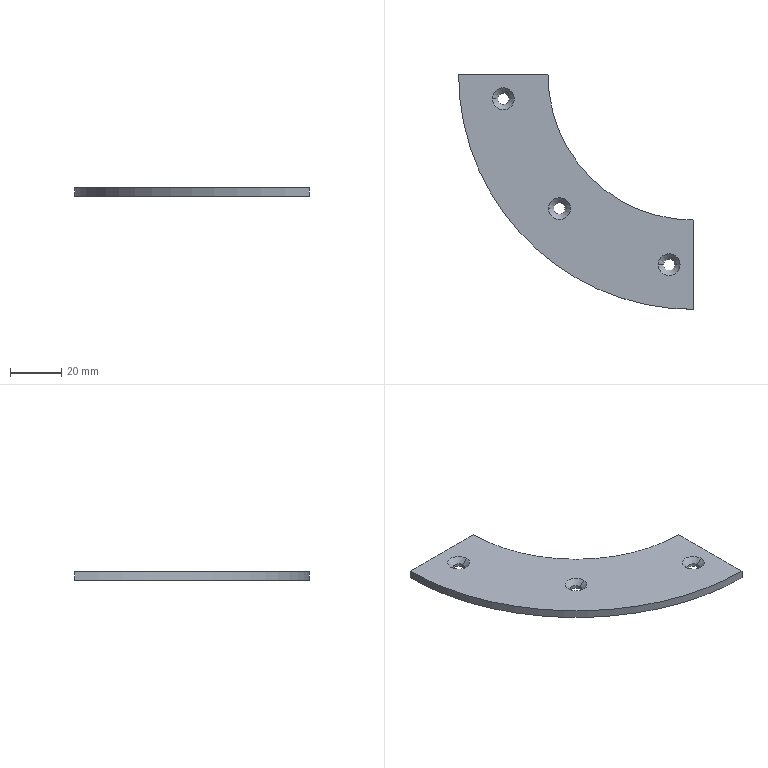Part | SolidWorks | features BaseBody 1 | 1 solid | 18 faces | box 92 x 92 x 3.2 mm | volume 12838 mm3 | cylinder 8 | cone 6 | plane 4 | commonest cylinder face diameters 4.5 x6 114 x1 184 x1
STEP:
#1=CARTESIAN_POINT('',(-50.25,-52.5,-3.2));
#2=VERTEX_POINT('',#1);
#3=CARTESIAN_POINT('',(-54.75,-52.5,-3.2));
#4=VERTEX_POINT('',#3);
#5=CARTESIAN_POINT('',(-52.5,-52.5,-3.2));
#6=DIRECTION('',(0.,0.,-1.));
#7=DIRECTION('',(1.,0.,0.));
#8=AXIS2_PLACEMENT_3D('',#5,#6,#7);
#9=CIRCLE('',#8,2.25);
#10=EDGE_CURVE('',#2,#4,#9,.T.);
#11=ORIENTED_EDGE('',*,*,#10,.T.);
#12=CARTESIAN_POINT('',(-54.75,-52.5,-2.05));
#13=VERTEX_POINT('',#12);
#14=CARTESIAN_POINT('',(-54.75,-52.5,0.));
#15=DIRECTION('',(0.,0.,1.));
#16=VECTOR('',#15,1000.);
#17=LINE('',#14,#16);
#18=EDGE_CURVE('',#4,#13,#17,.T.);
#19=ORIENTED_EDGE('',*,*,#18,.T.);
#20=CARTESIAN_POINT('',(-50.25,-52.5,-2.05));
#21=VERTEX_POINT('',#20);
#22=CARTESIAN_POINT('',(-52.5,-52.5,-2.05));
#23=DIRECTION('',(0.,0.,-1.));
#24=DIRECTION('',(1.,0.,0.));
#25=AXIS2_PLACEMENT_3D('',#22,#23,#24);
#26=CIRCLE('',#25,2.25);
#27=EDGE_CURVE('',#21,#13,#26,.T.);
#28=ORIENTED_EDGE('',*,*,#27,.F.);
#29=CARTESIAN_POINT('',(-50.25,-52.5,0.));
#30=DIRECTION('',(0.,0.,1.));
#31=VECTOR('',#30,1000.);
#32=LINE('',#29,#31);
#33=EDGE_CURVE('',#2,#21,#32,.T.);
#34=ORIENTED_EDGE('',*,*,#33,.F.);
#35=EDGE_LOOP('',(#11,#19,#28,#34));
#36=FACE_OUTER_BOUND('',#35,.T.);
#37=CARTESIAN_POINT('',(-52.5,-52.5,0.));
#38=DIRECTION('',(0.,0.,1.));
#39=DIRECTION('',(1.,0.,0.));
#40=AXIS2_PLACEMENT_3D('',#37,#38,#39);
#41=CYLINDRICAL_SURFACE('',#40,2.25);
#42=ADVANCED_FACE('',(#36),#41,.F.);
#43=CARTESIAN_POINT('',(-72.25,-9.5,-3.2));
#44=VERTEX_POINT('',#43);
#45=CARTESIAN_POINT('',(-76.75,-9.5,-3.2));
#46=VERTEX_POINT('',#45);
#47=CARTESIAN_POINT('',(-74.5,-9.5,-3.2));
#48=DIRECTION('',(0.,0.,-1.));
#49=DIRECTION('',(1.,0.,0.));
#50=AXIS2_PLACEMENT_3D('',#47,#48,#49);
#51=CIRCLE('',#50,2.25);
#52=EDGE_CURVE('',#44,#46,#51,.T.);
#53=ORIENTED_EDGE('',*,*,#52,.T.);
#54=CARTESIAN_POINT('',(-76.75,-9.5,-2.05));
#55=VERTEX_POINT('',#54);
#56=CARTESIAN_POINT('',(-76.75,-9.5,0.));
#57=DIRECTION('',(0.,0.,1.));
#58=VECTOR('',#57,1000.);
#59=LINE('',#56,#58);
#60=EDGE_CURVE('',#46,#55,#59,.T.);
#61=ORIENTED_EDGE('',*,*,#60,.T.);
#62=CARTESIAN_POINT('',(-72.25,-9.5,-2.05));
#63=VERTEX_POINT('',#62);
#64=CARTESIAN_POINT('',(-74.5,-9.5,-2.05));
#65=DIRECTION('',(0.,0.,-1.));
#66=DIRECTION('',(1.,0.,0.));
#67=AXIS2_PLACEMENT_3D('',#64,#65,#66);
#68=CIRCLE('',#67,2.25);
#69=EDGE_CURVE('',#63,#55,#68,.T.);
#70=ORIENTED_EDGE('',*,*,#69,.F.);
#71=CARTESIAN_POINT('',(-72.25,-9.5,0.));
#72=DIRECTION('',(0.,0.,1.));
#73=VECTOR('',#72,1000.);
#74=LINE('',#71,#73);
#75=EDGE_CURVE('',#44,#63,#74,.T.);
#76=ORIENTED_EDGE('',*,*,#75,.F.);
#77=EDGE_LOOP('',(#53,#61,#70,#76));
#78=FACE_OUTER_BOUND('',#77,.T.);
#79=CARTESIAN_POINT('',(-74.5,-9.5,0.));
#80=DIRECTION('',(0.,0.,1.));
#81=DIRECTION('',(1.,0.,0.));
#82=AXIS2_PLACEMENT_3D('',#79,#80,#81);
#83=CYLINDRICAL_SURFACE('',#82,2.25);
#84=ADVANCED_FACE('',(#78),#83,.F.);
#85=CARTESIAN_POINT('',(-7.25,-74.5,-3.2));
#86=VERTEX_POINT('',#85);
#87=CARTESIAN_POINT('',(-11.75,-74.5,-3.2));
#88=VERTEX_POINT('',#87);
#89=CARTESIAN_POINT('',(-9.5,-74.5,-3.2));
#90=DIRECTION('',(0.,0.,-1.));
#91=DIRECTION('',(1.,0.,0.));
#92=AXIS2_PLACEMENT_3D('',#89,#90,#91);
#93=CIRCLE('',#92,2.25);
#94=EDGE_CURVE('',#86,#88,#93,.T.);
#95=ORIENTED_EDGE('',*,*,#94,.T.);
#96=CARTESIAN_POINT('',(-11.75,-74.5,-2.05));
#97=VERTEX_POINT('',#96);
#98=CARTESIAN_POINT('',(-11.75,-74.5,0.));
#99=DIRECTION('',(0.,0.,1.));
#100=VECTOR('',#99,1000.);
#101=LINE('',#98,#100);
#102=EDGE_CURVE('',#88,#97,#101,.T.);
#103=ORIENTED_EDGE('',*,*,#102,.T.);
#104=CARTESIAN_POINT('',(-7.25,-74.5,-2.05));
#105=VERTEX_POINT('',#104);
#106=CARTESIAN_POINT('',(-9.5,-74.5,-2.05));
#107=DIRECTION('',(0.,0.,-1.));
#108=DIRECTION('',(1.,0.,0.));
#109=AXIS2_PLACEMENT_3D('',#106,#107,#108);
#110=CIRCLE('',#109,2.25);
#111=EDGE_CURVE('',#105,#97,#110,.T.);
#112=ORIENTED_EDGE('',*,*,#111,.F.);
#113=CARTESIAN_POINT('',(-7.25,-74.5,0.));
#114=DIRECTION('',(0.,0.,1.));
#115=VECTOR('',#114,1000.);
#116=LINE('',#113,#115);
#117=EDGE_CURVE('',#86,#105,#116,.T.);
#118=ORIENTED_EDGE('',*,*,#117,.F.);
#119=EDGE_LOOP('',(#95,#103,#112,#118));
#120=FACE_OUTER_BOUND('',#119,.T.);
#121=CARTESIAN_POINT('',(-9.5,-74.5,0.));
#122=DIRECTION('',(0.,0.,1.));
#123=DIRECTION('',(1.,0.,0.));
#124=AXIS2_PLACEMENT_3D('',#121,#122,#123);
#125=CYLINDRICAL_SURFACE('',#124,2.25);
#126=ADVANCED_FACE('',(#120),#125,.F.);
#127=ORIENTED_EDGE('',*,*,#27,.T.);
#128=CARTESIAN_POINT('',(-56.8,-52.5,0.));
#129=VERTEX_POINT('',#128);
#130=CARTESIAN_POINT('',(-56.8,-52.5,0.));
#131=DIRECTION('',(-0.7071,0.,0.7071));
#132=VECTOR('',#131,1000.);
#133=LINE('',#130,#132);
#134=EDGE_CURVE('',#13,#129,#133,.T.);
#135=ORIENTED_EDGE('',*,*,#134,.T.);
#136=CARTESIAN_POINT('',(-48.2,-52.5,0.));
#137=VERTEX_POINT('',#136);
#138=CARTESIAN_POINT('',(-52.5,-52.5,0.));
#139=DIRECTION('',(0.,0.,-1.));
#140=DIRECTION('',(1.,0.,0.));
#141=AXIS2_PLACEMENT_3D('',#138,#139,#140);
#142=CIRCLE('',#141,4.3);
#143=EDGE_CURVE('',#137,#129,#142,.T.);
#144=ORIENTED_EDGE('',*,*,#143,.F.);
#145=CARTESIAN_POINT('',(-48.2,-52.5,0.));
#146=DIRECTION('',(0.7071,0.,0.7071));
#147=VECTOR('',#146,1000.);
#148=LINE('',#145,#147);
#149=EDGE_CURVE('',#21,#137,#148,.T.);
#150=ORIENTED_EDGE('',*,*,#149,.F.);
#151=EDGE_LOOP('',(#127,#135,#144,#150));
#152=FACE_OUTER_BOUND('',#151,.T.);
#153=CARTESIAN_POINT('',(-52.5,-52.5,0.));
#154=DIRECTION('',(0.,0.,1.));
#155=DIRECTION('',(1.,0.,0.));
#156=AXIS2_PLACEMENT_3D('',#153,#154,#155);
#157=CONICAL_SURFACE('',#156,4.3,0.7854);
#158=ADVANCED_FACE('',(#152),#157,.F.);
#159=ORIENTED_EDGE('',*,*,#69,.T.);
#160=CARTESIAN_POINT('',(-78.8,-9.5,0.));
#161=VERTEX_POINT('',#160);
#162=CARTESIAN_POINT('',(-78.8,-9.5,0.));
#163=DIRECTION('',(-0.7071,0.,0.7071));
#164=VECTOR('',#163,1000.);
#165=LINE('',#162,#164);
#166=EDGE_CURVE('',#55,#161,#165,.T.);
#167=ORIENTED_EDGE('',*,*,#166,.T.);
#168=CARTESIAN_POINT('',(-70.2,-9.5,0.));
#169=VERTEX_POINT('',#168);
#170=CARTESIAN_POINT('',(-74.5,-9.5,0.));
#171=DIRECTION('',(0.,0.,-1.));
#172=DIRECTION('',(1.,0.,0.));
#173=AXIS2_PLACEMENT_3D('',#170,#171,#172);
#174=CIRCLE('',#173,4.3);
#175=EDGE_CURVE('',#169,#161,#174,.T.);
#176=ORIENTED_EDGE('',*,*,#175,.F.);
#177=CARTESIAN_POINT('',(-70.2,-9.5,0.));
#178=DIRECTION('',(0.7071,0.,0.7071));
#179=VECTOR('',#178,1000.);
#180=LINE('',#177,#179);
#181=EDGE_CURVE('',#63,#169,#180,.T.);
#182=ORIENTED_EDGE('',*,*,#181,.F.);
#183=EDGE_LOOP('',(#159,#167,#176,#182));
#184=FACE_OUTER_BOUND('',#183,.T.);
#185=CARTESIAN_POINT('',(-74.5,-9.5,0.));
#186=DIRECTION('',(0.,0.,1.));
#187=DIRECTION('',(1.,0.,0.));
#188=AXIS2_PLACEMENT_3D('',#185,#186,#187);
#189=CONICAL_SURFACE('',#188,4.3,0.7854);
#190=ADVANCED_FACE('',(#184),#189,.F.);
#191=ORIENTED_EDGE('',*,*,#111,.T.);
#192=CARTESIAN_POINT('',(-13.8,-74.5,0.));
#193=VERTEX_POINT('',#192);
#194=CARTESIAN_POINT('',(-13.8,-74.5,0.));
#195=DIRECTION('',(-0.7071,0.,0.7071));
#196=VECTOR('',#195,1000.);
#197=LINE('',#194,#196);
#198=EDGE_CURVE('',#97,#193,#197,.T.);
#199=ORIENTED_EDGE('',*,*,#198,.T.);
#200=CARTESIAN_POINT('',(-5.2,-74.5,0.));
#201=VERTEX_POINT('',#200);
#202=CARTESIAN_POINT('',(-9.5,-74.5,0.));
#203=DIRECTION('',(0.,0.,-1.));
#204=DIRECTION('',(1.,0.,0.));
#205=AXIS2_PLACEMENT_3D('',#202,#203,#204);
#206=CIRCLE('',#205,4.3);
#207=EDGE_CURVE('',#201,#193,#206,.T.);
#208=ORIENTED_EDGE('',*,*,#207,.F.);
#209=CARTESIAN_POINT('',(-5.2,-74.5,0.));
#210=DIRECTION('',(0.7071,0.,0.7071));
#211=VECTOR('',#210,1000.);
#212=LINE('',#209,#211);
#213=EDGE_CURVE('',#105,#201,#212,.T.);
#214=ORIENTED_EDGE('',*,*,#213,.F.);
#215=EDGE_LOOP('',(#191,#199,#208,#214));
#216=FACE_OUTER_BOUND('',#215,.T.);
#217=CARTESIAN_POINT('',(-9.5,-74.5,0.));
#218=DIRECTION('',(0.,0.,1.));
#219=DIRECTION('',(1.,0.,0.));
#220=AXIS2_PLACEMENT_3D('',#217,#218,#219);
#221=CONICAL_SURFACE('',#220,4.3,0.7854);
#222=ADVANCED_FACE('',(#216),#221,.F.);
#223=CARTESIAN_POINT('',(0.,-92.,-3.2));
#224=VERTEX_POINT('',#223);
#225=CARTESIAN_POINT('',(0.,-57.,-3.2));
#226=VERTEX_POINT('',#225);
#227=CARTESIAN_POINT('',(0.,0.,-3.2));
#228=DIRECTION('',(0.,1.,0.));
#229=VECTOR('',#228,1000.);
#230=LINE('',#227,#229);
#231=EDGE_CURVE('',#224,#226,#230,.T.);
#232=ORIENTED_EDGE('',*,*,#231,.F.);
#233=CARTESIAN_POINT('',(-92.,0.,-3.2));
#234=VERTEX_POINT('',#233);
#235=CARTESIAN_POINT('',(0.,0.,-3.2));
#236=DIRECTION('',(0.,0.,1.));
#237=DIRECTION('',(1.,0.,0.));
#238=AXIS2_PLACEMENT_3D('',#235,#236,#237);
#239=CIRCLE('',#238,92.);
#240=EDGE_CURVE('',#234,#224,#239,.T.);
#241=ORIENTED_EDGE('',*,*,#240,.F.);
#242=CARTESIAN_POINT('',(-57.,0.,-3.2));
#243=VERTEX_POINT('',#242);
#244=CARTESIAN_POINT('',(0.,0.,-3.2));
#245=DIRECTION('',(-1.,0.,0.));
#246=VECTOR('',#245,1000.);
#247=LINE('',#244,#246);
#248=EDGE_CURVE('',#243,#234,#247,.T.);
#249=ORIENTED_EDGE('',*,*,#248,.F.);
#250=CARTESIAN_POINT('',(0.,0.,-3.2));
#251=DIRECTION('',(0.,0.,-1.));
#252=DIRECTION('',(1.,0.,0.));
#253=AXIS2_PLACEMENT_3D('',#250,#251,#252);
#254=CIRCLE('',#253,57.);
#255=EDGE_CURVE('',#226,#243,#254,.T.);
#256=ORIENTED_EDGE('',*,*,#255,.F.);
#257=EDGE_LOOP('',(#232,#241,#249,#256));
#258=FACE_OUTER_BOUND('',#257,.T.);
#259=ORIENTED_EDGE('',*,*,#10,.F.);
#260=CARTESIAN_POINT('',(-52.5,-52.5,-3.2));
#261=DIRECTION('',(0.,0.,-1.));
#262=DIRECTION('',(1.,0.,0.));
#263=AXIS2_PLACEMENT_3D('',#260,#261,#262);
#264=CIRCLE('',#263,2.25);
#265=EDGE_CURVE('',#4,#2,#264,.T.);
#266=ORIENTED_EDGE('',*,*,#265,.F.);
#267=EDGE_LOOP('',(#259,#266));
#268=FACE_BOUND('',#267,.T.);
#269=ORIENTED_EDGE('',*,*,#52,.F.);
#270=CARTESIAN_POINT('',(-74.5,-9.5,-3.2));
#271=DIRECTION('',(0.,0.,-1.));
#272=DIRECTION('',(1.,0.,0.));
#273=AXIS2_PLACEMENT_3D('',#270,#271,#272);
#274=CIRCLE('',#273,2.25);
#275=EDGE_CURVE('',#46,#44,#274,.T.);
#276=ORIENTED_EDGE('',*,*,#275,.F.);
#277=EDGE_LOOP('',(#269,#276));
#278=FACE_BOUND('',#277,.T.);
#279=ORIENTED_EDGE('',*,*,#94,.F.);
#280=CARTESIAN_POINT('',(-9.5,-74.5,-3.2));
#281=DIRECTION('',(0.,0.,-1.));
#282=DIRECTION('',(1.,0.,0.));
#283=AXIS2_PLACEMENT_3D('',#280,#281,#282);
#284=CIRCLE('',#283,2.25);
#285=EDGE_CURVE('',#88,#86,#284,.T.);
#286=ORIENTED_EDGE('',*,*,#285,.F.);
#287=EDGE_LOOP('',(#279,#286));
#288=FACE_BOUND('',#287,.T.);
#289=CARTESIAN_POINT('',(0.,0.,-3.2));
#290=DIRECTION('',(0.,0.,1.));
#291=DIRECTION('',(1.,0.,0.));
#292=AXIS2_PLACEMENT_3D('',#289,#290,#291);
#293=PLANE('',#292);
#294=ADVANCED_FACE('',(#258,#268,#278,#288),#293,.F.);
#295=CARTESIAN_POINT('',(0.,-57.,0.));
#296=VERTEX_POINT('',#295);
#297=CARTESIAN_POINT('',(0.,-57.,-3.2));
#298=DIRECTION('',(0.,0.,1.));
#299=VECTOR('',#298,1000.);
#300=LINE('',#297,#299);
#301=EDGE_CURVE('',#226,#296,#300,.T.);
#302=ORIENTED_EDGE('',*,*,#301,.F.);
#303=ORIENTED_EDGE('',*,*,#255,.T.);
#304=CARTESIAN_POINT('',(-57.,0.,0.));
#305=VERTEX_POINT('',#304);
#306=CARTESIAN_POINT('',(-57.,0.,-3.2));
#307=DIRECTION('',(0.,0.,-1.));
#308=VECTOR('',#307,1000.);
#309=LINE('',#306,#308);
#310=EDGE_CURVE('',#305,#243,#309,.T.);
#311=ORIENTED_EDGE('',*,*,#310,.F.);
#312=CARTESIAN_POINT('',(0.,0.,0.));
#313=DIRECTION('',(0.,0.,-1.));
#314=DIRECTION('',(1.,0.,0.));
#315=AXIS2_PLACEMENT_3D('',#312,#313,#314);
#316=CIRCLE('',#315,57.);
#317=EDGE_CURVE('',#296,#305,#316,.T.);
#318=ORIENTED_EDGE('',*,*,#317,.F.);
#319=EDGE_LOOP('',(#302,#303,#311,#318));
#320=FACE_OUTER_BOUND('',#319,.T.);
#321=CARTESIAN_POINT('',(0.,0.,-3.2));
#322=DIRECTION('',(0.,0.,1.));
#323=DIRECTION('',(1.,0.,0.));
#324=AXIS2_PLACEMENT_3D('',#321,#322,#323);
#325=CYLINDRICAL_SURFACE('',#324,57.);
#326=ADVANCED_FACE('',(#320),#325,.F.);
#327=ORIENTED_EDGE('',*,*,#231,.T.);
#328=ORIENTED_EDGE('',*,*,#301,.T.);
#329=CARTESIAN_POINT('',(0.,-92.,0.));
#330=VERTEX_POINT('',#329);
#331=CARTESIAN_POINT('',(0.,-57.,0.));
#332=DIRECTION('',(0.,-1.,0.));
#333=VECTOR('',#332,1000.);
#334=LINE('',#331,#333);
#335=EDGE_CURVE('',#296,#330,#334,.T.);
#336=ORIENTED_EDGE('',*,*,#335,.T.);
#337=CARTESIAN_POINT('',(0.,-92.,-3.2));
#338=DIRECTION('',(0.,0.,-1.));
#339=VECTOR('',#338,1000.);
#340=LINE('',#337,#339);
#341=EDGE_CURVE('',#330,#224,#340,.T.);
#342=ORIENTED_EDGE('',*,*,#341,.T.);
#343=EDGE_LOOP('',(#327,#328,#336,#342));
#344=FACE_OUTER_BOUND('',#343,.T.);
#345=CARTESIAN_POINT('',(0.,-57.,-3.2));
#346=DIRECTION('',(1.,0.,0.));
#347=DIRECTION('',(0.,0.,-1.));
#348=AXIS2_PLACEMENT_3D('',#345,#346,#347);
#349=PLANE('',#348);
#350=ADVANCED_FACE('',(#344),#349,.T.);
#351=ORIENTED_EDGE('',*,*,#240,.T.);
#352=ORIENTED_EDGE('',*,*,#341,.F.);
#353=CARTESIAN_POINT('',(-92.,0.,0.));
#354=VERTEX_POINT('',#353);
#355=CARTESIAN_POINT('',(0.,0.,0.));
#356=DIRECTION('',(0.,0.,-1.));
#357=DIRECTION('',(1.,0.,0.));
#358=AXIS2_PLACEMENT_3D('',#355,#356,#357);
#359=CIRCLE('',#358,92.);
#360=EDGE_CURVE('',#330,#354,#359,.T.);
#361=ORIENTED_EDGE('',*,*,#360,.T.);
#362=CARTESIAN_POINT('',(-92.,0.,-3.2));
#363=DIRECTION('',(0.,0.,-1.));
#364=VECTOR('',#363,1000.);
#365=LINE('',#362,#364);
#366=EDGE_CURVE('',#354,#234,#365,.T.);
#367=ORIENTED_EDGE('',*,*,#366,.T.);
#368=EDGE_LOOP('',(#351,#352,#361,#367));
#369=FACE_OUTER_BOUND('',#368,.T.);
#370=CARTESIAN_POINT('',(0.,0.,-3.2));
#371=DIRECTION('',(0.,0.,1.));
#372=DIRECTION('',(1.,0.,0.));
#373=AXIS2_PLACEMENT_3D('',#370,#371,#372);
#374=CYLINDRICAL_SURFACE('',#373,92.);
#375=ADVANCED_FACE('',(#369),#374,.T.);
#376=ORIENTED_EDGE('',*,*,#248,.T.);
#377=ORIENTED_EDGE('',*,*,#366,.F.);
#378=CARTESIAN_POINT('',(-57.,0.,0.));
#379=DIRECTION('',(1.,0.,0.));
#380=VECTOR('',#379,1000.);
#381=LINE('',#378,#380);
#382=EDGE_CURVE('',#354,#305,#381,.T.);
#383=ORIENTED_EDGE('',*,*,#382,.T.);
#384=ORIENTED_EDGE('',*,*,#310,.T.);
#385=EDGE_LOOP('',(#376,#377,#383,#384));
#386=FACE_OUTER_BOUND('',#385,.T.);
#387=CARTESIAN_POINT('',(-57.,0.,-3.2));
#388=DIRECTION('',(0.,1.,0.));
#389=DIRECTION('',(0.,0.,1.));
#390=AXIS2_PLACEMENT_3D('',#387,#388,#389);
#391=PLANE('',#390);
#392=ADVANCED_FACE('',(#386),#391,.T.);
#393=ORIENTED_EDGE('',*,*,#18,.F.);
#394=ORIENTED_EDGE('',*,*,#265,.T.);
#395=ORIENTED_EDGE('',*,*,#33,.T.);
#396=CARTESIAN_POINT('',(-52.5,-52.5,-2.05));
#397=DIRECTION('',(0.,0.,-1.));
#398=DIRECTION('',(1.,0.,0.));
#399=AXIS2_PLACEMENT_3D('',#396,#397,#398);
#400=CIRCLE('',#399,2.25);
#401=EDGE_CURVE('',#13,#21,#400,.T.);
#402=ORIENTED_EDGE('',*,*,#401,.F.);
#403=EDGE_LOOP('',(#393,#394,#395,#402));
#404=FACE_OUTER_BOUND('',#403,.T.);
#405=CARTESIAN_POINT('',(-52.5,-52.5,0.));
#406=DIRECTION('',(0.,0.,1.));
#407=DIRECTION('',(1.,0.,0.));
#408=AXIS2_PLACEMENT_3D('',#405,#406,#407);
#409=CYLINDRICAL_SURFACE('',#408,2.25);
#410=ADVANCED_FACE('',(#404),#409,.F.);
#411=ORIENTED_EDGE('',*,*,#60,.F.);
#412=ORIENTED_EDGE('',*,*,#275,.T.);
#413=ORIENTED_EDGE('',*,*,#75,.T.);
#414=CARTESIAN_POINT('',(-74.5,-9.5,-2.05));
#415=DIRECTION('',(0.,0.,-1.));
#416=DIRECTION('',(1.,0.,0.));
#417=AXIS2_PLACEMENT_3D('',#414,#415,#416);
#418=CIRCLE('',#417,2.25);
#419=EDGE_CURVE('',#55,#63,#418,.T.);
#420=ORIENTED_EDGE('',*,*,#419,.F.);
#421=EDGE_LOOP('',(#411,#412,#413,#420));
#422=FACE_OUTER_BOUND('',#421,.T.);
#423=CARTESIAN_POINT('',(-74.5,-9.5,0.));
#424=DIRECTION('',(0.,0.,1.));
#425=DIRECTION('',(1.,0.,0.));
#426=AXIS2_PLACEMENT_3D('',#423,#424,#425);
#427=CYLINDRICAL_SURFACE('',#426,2.25);
#428=ADVANCED_FACE('',(#422),#427,.F.);
#429=ORIENTED_EDGE('',*,*,#102,.F.);
#430=ORIENTED_EDGE('',*,*,#285,.T.);
#431=ORIENTED_EDGE('',*,*,#117,.T.);
#432=CARTESIAN_POINT('',(-9.5,-74.5,-2.05));
#433=DIRECTION('',(0.,0.,-1.));
#434=DIRECTION('',(1.,0.,0.));
#435=AXIS2_PLACEMENT_3D('',#432,#433,#434);
#436=CIRCLE('',#435,2.25);
#437=EDGE_CURVE('',#97,#105,#436,.T.);
#438=ORIENTED_EDGE('',*,*,#437,.F.);
#439=EDGE_LOOP('',(#429,#430,#431,#438));
#440=FACE_OUTER_BOUND('',#439,.T.);
#441=CARTESIAN_POINT('',(-9.5,-74.5,0.));
#442=DIRECTION('',(0.,0.,1.));
#443=DIRECTION('',(1.,0.,0.));
#444=AXIS2_PLACEMENT_3D('',#441,#442,#443);
#445=CYLINDRICAL_SURFACE('',#444,2.25);
#446=ADVANCED_FACE('',(#440),#445,.F.);
#447=ORIENTED_EDGE('',*,*,#360,.F.);
#448=ORIENTED_EDGE('',*,*,#335,.F.);
#449=ORIENTED_EDGE('',*,*,#317,.T.);
#450=ORIENTED_EDGE('',*,*,#382,.F.);
#451=EDGE_LOOP('',(#447,#448,#449,#450));
#452=FACE_OUTER_BOUND('',#451,.T.);
#453=ORIENTED_EDGE('',*,*,#143,.T.);
#454=CARTESIAN_POINT('',(-52.5,-52.5,0.));
#455=DIRECTION('',(0.,0.,-1.));
#456=DIRECTION('',(1.,0.,0.));
#457=AXIS2_PLACEMENT_3D('',#454,#455,#456);
#458=CIRCLE('',#457,4.3);
#459=EDGE_CURVE('',#129,#137,#458,.T.);
#460=ORIENTED_EDGE('',*,*,#459,.T.);
#461=EDGE_LOOP('',(#453,#460));
#462=FACE_BOUND('',#461,.T.);
#463=ORIENTED_EDGE('',*,*,#175,.T.);
#464=CARTESIAN_POINT('',(-74.5,-9.5,0.));
#465=DIRECTION('',(0.,0.,-1.));
#466=DIRECTION('',(1.,0.,0.));
#467=AXIS2_PLACEMENT_3D('',#464,#465,#466);
#468=CIRCLE('',#467,4.3);
#469=EDGE_CURVE('',#161,#169,#468,.T.);
#470=ORIENTED_EDGE('',*,*,#469,.T.);
#471=EDGE_LOOP('',(#463,#470));
#472=FACE_BOUND('',#471,.T.);
#473=ORIENTED_EDGE('',*,*,#207,.T.);
#474=CARTESIAN_POINT('',(-9.5,-74.5,0.));
#475=DIRECTION('',(0.,0.,-1.));
#476=DIRECTION('',(1.,0.,0.));
#477=AXIS2_PLACEMENT_3D('',#474,#475,#476);
#478=CIRCLE('',#477,4.3);
#479=EDGE_CURVE('',#193,#201,#478,.T.);
#480=ORIENTED_EDGE('',*,*,#479,.T.);
#481=EDGE_LOOP('',(#473,#480));
#482=FACE_BOUND('',#481,.T.);
#483=CARTESIAN_POINT('',(0.,0.,0.));
#484=DIRECTION('',(0.,0.,1.));
#485=DIRECTION('',(1.,0.,0.));
#486=AXIS2_PLACEMENT_3D('',#483,#484,#485);
#487=PLANE('',#486);
#488=ADVANCED_FACE('',(#452,#462,#472,#482),#487,.T.);
#489=ORIENTED_EDGE('',*,*,#134,.F.);
#490=ORIENTED_EDGE('',*,*,#401,.T.);
#491=ORIENTED_EDGE('',*,*,#149,.T.);
#492=ORIENTED_EDGE('',*,*,#459,.F.);
#493=EDGE_LOOP('',(#489,#490,#491,#492));
#494=FACE_OUTER_BOUND('',#493,.T.);
#495=CARTESIAN_POINT('',(-52.5,-52.5,0.));
#496=DIRECTION('',(0.,0.,1.));
#497=DIRECTION('',(1.,0.,0.));
#498=AXIS2_PLACEMENT_3D('',#495,#496,#497);
#499=CONICAL_SURFACE('',#498,4.3,0.7854);
#500=ADVANCED_FACE('',(#494),#499,.F.);
#501=ORIENTED_EDGE('',*,*,#166,.F.);
#502=ORIENTED_EDGE('',*,*,#419,.T.);
#503=ORIENTED_EDGE('',*,*,#181,.T.);
#504=ORIENTED_EDGE('',*,*,#469,.F.);
#505=EDGE_LOOP('',(#501,#502,#503,#504));
#506=FACE_OUTER_BOUND('',#505,.T.);
#507=CARTESIAN_POINT('',(-74.5,-9.5,0.));
#508=DIRECTION('',(0.,0.,1.));
#509=DIRECTION('',(1.,0.,0.));
#510=AXIS2_PLACEMENT_3D('',#507,#508,#509);
#511=CONICAL_SURFACE('',#510,4.3,0.7854);
#512=ADVANCED_FACE('',(#506),#511,.F.);
#513=ORIENTED_EDGE('',*,*,#198,.F.);
#514=ORIENTED_EDGE('',*,*,#437,.T.);
#515=ORIENTED_EDGE('',*,*,#213,.T.);
#516=ORIENTED_EDGE('',*,*,#479,.F.);
#517=EDGE_LOOP('',(#513,#514,#515,#516));
#518=FACE_OUTER_BOUND('',#517,.T.);
#519=CARTESIAN_POINT('',(-9.5,-74.5,0.));
#520=DIRECTION('',(0.,0.,1.));
#521=DIRECTION('',(1.,0.,0.));
#522=AXIS2_PLACEMENT_3D('',#519,#520,#521);
#523=CONICAL_SURFACE('',#522,4.3,0.7854);
#524=ADVANCED_FACE('',(#518),#523,.F.);
#525=CLOSED_SHELL('',(#42,#84,#126,#158,#190,#222,#294,#326,#350,#375,#392,#410,#428,#446,#488,#500,#512,#524));
#526=MANIFOLD_SOLID_BREP('',#525);
#527=CARTESIAN_POINT('',(0.,0.,0.));
#528=DIRECTION('',(0.,0.,1.));
#529=DIRECTION('',(1.,0.,0.));
#530=AXIS2_PLACEMENT_3D('',#527,#528,#529);
#531=(LENGTH_UNIT()NAMED_UNIT(*)SI_UNIT(.MILLI.,.METRE.));
#532=UNCERTAINTY_MEASURE_WITH_UNIT(LENGTH_MEASURE(0.00001),#531,'','');
#533=(NAMED_UNIT(*)PLANE_ANGLE_UNIT()SI_UNIT($,.RADIAN.));
#534=(NAMED_UNIT(*)SI_UNIT($,.STERADIAN.)SOLID_ANGLE_UNIT());
#535=(GEOMETRIC_REPRESENTATION_CONTEXT(3)GLOBAL_UNCERTAINTY_ASSIGNED_CONTEXT((#532))GLOBAL_UNIT_ASSIGNED_CONTEXT((#531,#533,#534))REPRESENTATION_CONTEXT('',''));
#536=ADVANCED_BREP_SHAPE_REPRESENTATION('',(#526,#530),#535);